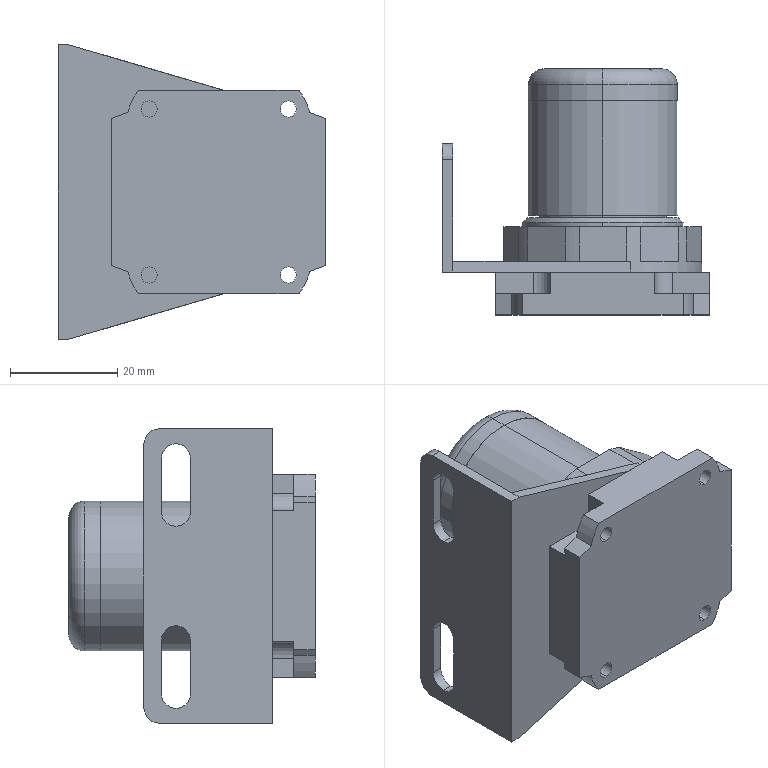Part | NX | features BREP 1 | 1 solid | 100 faces | box 50 x 46 x 55 mm | volume 41458 mm3 | plane 58 | cylinder 38 | torus 2 | cone 2 | commonest cylinder face diameters 3 x8 5.4 x6 37 x6 6.5 x4 24 x4 6 x2